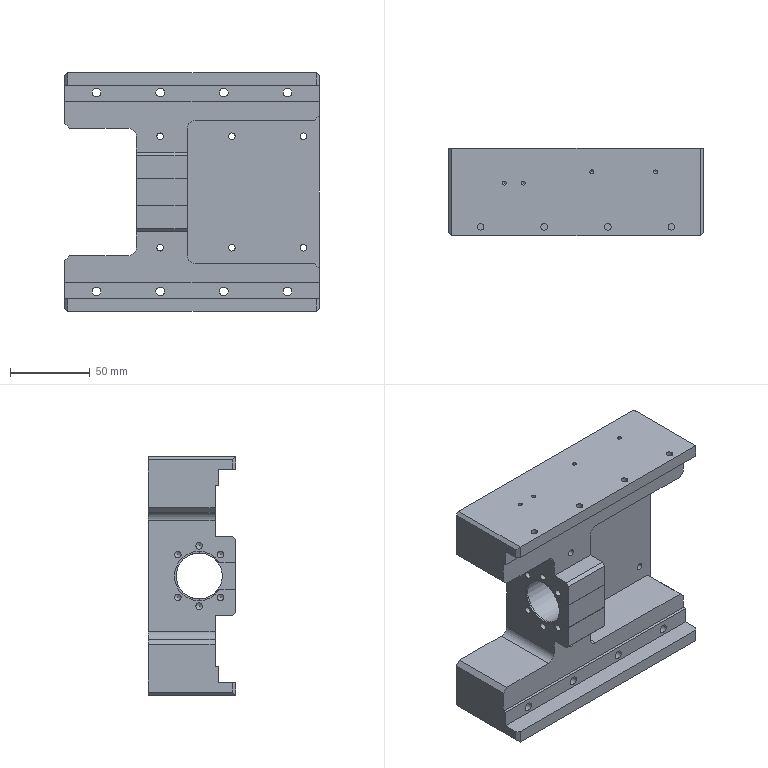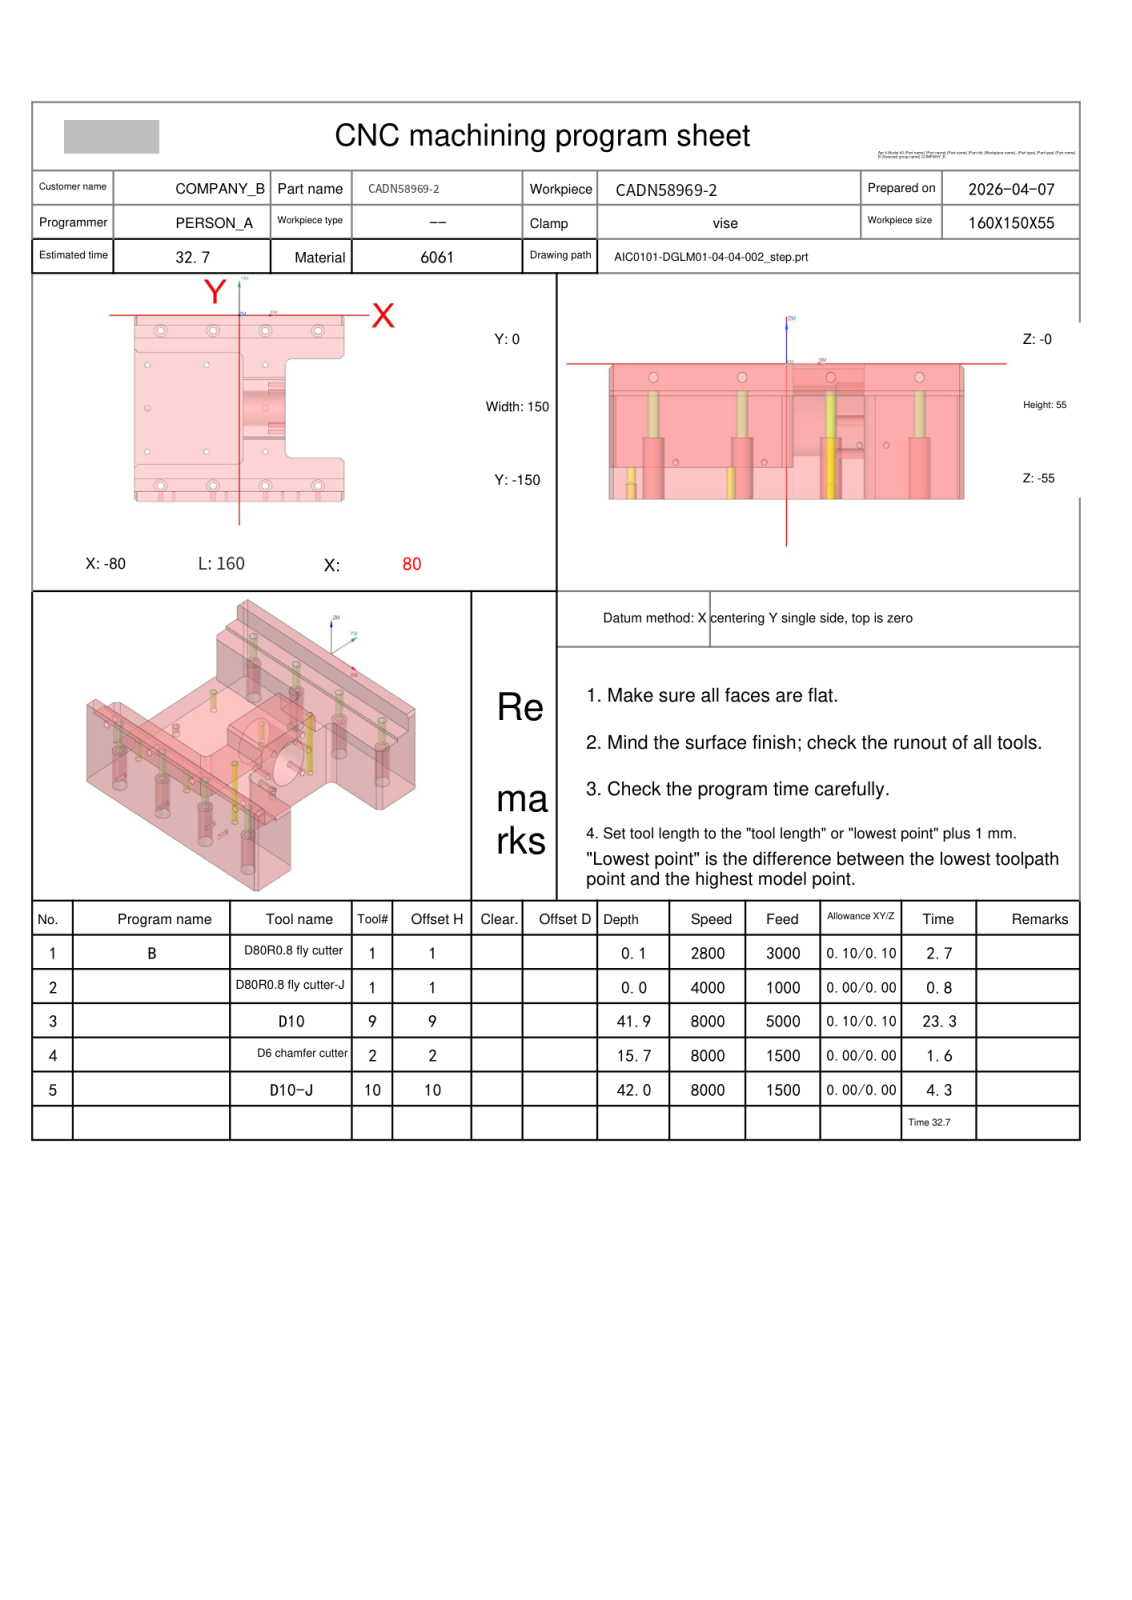NC program | NX | posted by the shop | part box 160 x 55 x 150 mm
Lines 13375 to 14160 of 14160:
N4 T02 M06
(D6 chamfer cutter D=6. R=0. H=02 ce=0.00 di=0.10)
G00 G90 G54 X20. Y-110. M03 S8000
G43 H02 Z20.
M08
G98 G81 X20. Y-110. Z-15.7 R-10. F1000.
Y-40.
G80
G00 Z20.
G00 G90 X78.792 Y-8.99 M03 S6500
Z20.
Z.13
G01 Z-1.2 F1500.
G03 X78.452 Y-8.915 I-.601 J-1.907
G01 X78.398 Y-8.905
X78.349 Y-8.928
X78.259 Y-8.966
X78. Y-9.
X-78.
X-78.259 Y-8.966
X-78.349 Y-8.929
X-78.398 Y-8.905
X-78.452 Y-8.915
G03 X-78.792 Y-8.991 I.261 J-1.983
G01 Z.13
G00 Z2.8
X-78.903 Y.41
G01 Z-1.2
X-78.866 Y.5
X-78.707 Y.707
X-78.5 Y.866
X-78.259 Y.966
X-78. Y1.
X0.0
X78.
X78.259 Y.966
X78.5 Y.866
X78.707 Y.707
X78.866 Y.5
X78.903 Y.41
Z2.8
G00 Z10.
X35.99 Y-51.208
Z.13
G01 Z-1.2
G03 X35.915 Y-51.548 I1.907 J-.601
G01 X35.905 Y-51.602
X35.928 Y-51.651
X35.966 Y-51.741
X36. Y-52.
Y-98.
X35.966 Y-98.259
X35.928 Y-98.349
X35.905 Y-98.398
X35.915 Y-98.452
G03 X35.99 Y-98.792 I1.983 J.261
G01 Z.13
G00 Z10.
X2.01
Z.13
G01 Z-1.2
G03 X2.085 Y-98.452 I-1.907 J.601
G01 X2.095 Y-98.398
X2.072 Y-98.349
X2.034 Y-98.259
X2. Y-98.
Y-75.
Y-52.
X2.034 Y-51.741
X2.072 Y-51.651
X2.095 Y-51.602
X2.085 Y-51.548
G03 X2.01 Y-51.208 I-1.983 J-.261
G01 Z.13
G00 Z10.
X78.903 Y-150.41
Z2.8
G01 Z-1.2
X78.866 Y-150.5
X78.707 Y-150.707
X78.5 Y-150.866
X78.259 Y-150.966
X78. Y-151.
X-78.
X-78.259 Y-150.966
X-78.5 Y-150.866
X-78.707 Y-150.707
X-78.866 Y-150.5
X-78.903 Y-150.41
Z2.8
G00 X-78.792 Y-141.01
Z.13
G01 Z-1.2
G03 X-78.452 Y-141.085 I.601 J1.907
G01 X-78.398 Y-141.095
X-78.349 Y-141.072
X-78.259 Y-141.034
X-78. Y-141.
X0.0
X78.
X78.259 Y-141.034
X78.349 Y-141.072
X78.398 Y-141.095
X78.452 Y-141.085
G03 X78.792 Y-141.01 I-.261 J1.983
G01 Z.13
G00 Z10.
X-81.068 Y-138.968
Z-2.305
G01 Z-12.2
X-81.008 Y-138.882
X-81. Y-138.852
Y-131.8
G02 X-80. Y-130.8 I1. J0.0
G01 X80.
G02 X81. Y-131.8 I0.0 J-1.
G01 Y-138.882
X81.005 Y-138.902
X81.045 Y-138.959
Z-2.292
G00 Z10.
X-59.172 Y-138.791
Z-1.81
G01 Z-12.2
G03 X-58.826 Y-138.749 I-.07 J1.999
G01 X-58.772 Y-138.74
X-58.733 Y-138.702
X-58.699 Y-138.671
G03 X-58.25 Y-137.5 I-1.301 J1.171
X-60. Y-135.75 I-1.75 J0.0
X-61.75 Y-137.5 I0.0 J-1.75
X-61.664 Y-138.041 I1.75 J0.0
G01 X-61.516 Y-138.375
X-61.301 Y-138.671
X-61.267 Y-138.702
X-61.232 Y-138.726
X-61.189 Y-138.76
X-61.135 Y-138.763
X-60.94 Y-138.772
X-60.786 Y-138.766
Z-1.835
G00 Z10.
X-19.172 Y-138.791
Z-1.81
G01 Z-12.2
G03 X-18.826 Y-138.749 I-.07 J1.999
G01 X-18.772 Y-138.74
X-18.733 Y-138.702
X-18.699 Y-138.671
G03 X-18.25 Y-137.5 I-1.301 J1.171
X-20. Y-135.75 I-1.75 J0.0
X-21.75 Y-137.5 I0.0 J-1.75
X-21.664 Y-138.041 I1.75 J0.0
G01 X-21.516 Y-138.375
X-21.301 Y-138.671
X-21.267 Y-138.702
X-21.232 Y-138.726
X-21.189 Y-138.76
X-21.135 Y-138.763
X-20.94 Y-138.772
X-20.786 Y-138.766
Z-1.835
G00 Z10.
X20.828 Y-138.791
Z-1.81
G01 Z-12.2
G03 X21.174 Y-138.749 I-.07 J1.999
G01 X21.228 Y-138.74
X21.267 Y-138.702
X21.301 Y-138.671
G03 X21.75 Y-137.5 I-1.301 J1.171
X20. Y-135.75 I-1.75 J0.0
X18.25 Y-137.5 I0.0 J-1.75
X18.336 Y-138.041 I1.75 J0.0
G01 X18.484 Y-138.375
X18.699 Y-138.671
X18.733 Y-138.702
X18.768 Y-138.726
X18.811 Y-138.76
X18.865 Y-138.763
X19.06 Y-138.772
X19.214 Y-138.766
Z-1.835
G00 Z10.
X60.828 Y-138.791
Z-1.81
G01 Z-12.2
G03 X61.174 Y-138.749 I-.07 J1.999
G01 X61.228 Y-138.74
X61.267 Y-138.702
X61.301 Y-138.671
G03 X61.75 Y-137.5 I-1.301 J1.171
X60. Y-135.75 I-1.75 J0.0
X58.25 Y-137.5 I0.0 J-1.75
X58.336 Y-138.041 I1.75 J0.0
G01 X58.484 Y-138.375
X58.699 Y-138.671
X58.733 Y-138.702
X58.768 Y-138.726
X58.811 Y-138.76
X58.865 Y-138.763
X59.06 Y-138.772
X59.214 Y-138.766
Z-1.835
G00 Z10.
X81.068 Y-11.032
Z-2.305
G01 Z-12.2
X81.008 Y-11.118
X81. Y-11.148
Y-18.2
G02 X80. Y-19.2 I-1. J0.0
G01 X-80.
G02 X-81. Y-18.2 I0.0 J1.
G01 Y-11.118
X-81.005 Y-11.098
X-81.045 Y-11.041
Z-2.292
G00 Z10.
X-60.828 Y-11.209
Z-1.81
G01 Z-12.2
G03 X-61.174 Y-11.251 I.07 J-1.999
G01 X-61.228 Y-11.26
X-61.267 Y-11.298
X-61.301 Y-11.329
G03 X-61.75 Y-12.5 I1.301 J-1.171
X-60. Y-14.25 I1.75 J0.0
X-58.25 Y-12.5 I0.0 J1.75
X-58.336 Y-11.959 I-1.75 J0.0
G01 X-58.484 Y-11.625
X-58.699 Y-11.329
X-58.733 Y-11.298
X-58.768 Y-11.274
X-58.811 Y-11.24
X-58.865 Y-11.237
X-59.06 Y-11.228
X-59.214 Y-11.234
Z-1.835
G00 Z10.
X-20.828 Y-11.209
Z-1.81
G01 Z-12.2
G03 X-21.174 Y-11.251 I.07 J-1.999
G01 X-21.228 Y-11.26
X-21.267 Y-11.298
X-21.301 Y-11.329
G03 X-21.75 Y-12.5 I1.301 J-1.171
X-20. Y-14.25 I1.75 J0.0
X-18.25 Y-12.5 I0.0 J1.75
X-18.336 Y-11.959 I-1.75 J0.0
G01 X-18.484 Y-11.625
X-18.699 Y-11.329
X-18.733 Y-11.298
X-18.768 Y-11.274
X-18.811 Y-11.24
X-18.865 Y-11.237
X-19.06 Y-11.228
X-19.214 Y-11.234
Z-1.835
G00 Z10.
X19.172 Y-11.209
Z-1.81
G01 Z-12.2
G03 X18.826 Y-11.251 I.07 J-1.999
G01 X18.772 Y-11.26
X18.733 Y-11.298
X18.699 Y-11.329
G03 X18.25 Y-12.5 I1.301 J-1.171
X20. Y-14.25 I1.75 J0.0
X21.75 Y-12.5 I0.0 J1.75
X21.664 Y-11.959 I-1.75 J0.0
G01 X21.516 Y-11.625
X21.301 Y-11.329
X21.267 Y-11.298
X21.232 Y-11.274
X21.189 Y-11.24
X21.135 Y-11.237
X20.94 Y-11.228
X20.786 Y-11.234
Z-1.835
G00 Z10.
X59.172 Y-11.209
Z-1.81
G01 Z-12.2
G03 X58.826 Y-11.251 I.07 J-1.999
G01 X58.772 Y-11.26
X58.733 Y-11.298
X58.699 Y-11.329
G03 X58.25 Y-12.5 I1.301 J-1.171
X59.636 Y-14.212 I1.75 J0.0
G01 X60. Y-14.25
G03 X61.75 Y-12.5 I0.0 J1.75
X61.516 Y-11.625 I-1.75 J0.0
G01 X61.301 Y-11.329
X61.267 Y-11.298
X61.232 Y-11.274
X61.189 Y-11.24
X61.135 Y-11.237
X60.94 Y-11.228
X60.786 Y-11.234
Z-1.835
G00 Z10.
X36.068 Y-103.009
Z-3.086
G01 Z-14.2
X36.008 Y-103.095
X36. Y-103.125
Y-110.
G03 X40. Y-114. I4. J0.0
G01 X77.
X77.259 Y-114.034
X77.5 Y-114.134
X77.707 Y-114.293
X80.707 Y-117.293
X80.866 Y-117.5
X80.966 Y-117.741
X81. Y-118.
Y-128.7
X81.008 Y-128.73
X81.068 Y-128.816
Z-12.669
G00 Z10.
X-81.068 Y-128.822
Z-12.669
G01 Z-14.2
X-81.008 Y-128.736
X-81. Y-128.706
Y-123.
X-80.966 Y-122.741
X-80.866 Y-122.5
X-80.707 Y-122.293
X-77.707 Y-119.293
X-77.5 Y-119.134
X-77.259 Y-119.034
X-77. Y-119.
X-2.
G03 X2. Y-115. I0.0 J4.
G01 Y-103.135
X1.992 Y-103.105
X1.932 Y-103.019
Z-3.096
G00 Z10.
X19.588 Y-110.926
Z-12.68
G01 Z-14.2
G03 X19.897 Y-111.086 I1.075 J1.687
G01 X19.946 Y-111.11
X20. Y-111.1
G03 X21.1 Y-110. I0.0 J1.1
X20. Y-108.9 I-1.1 J0.0
X18.9 Y-110. I0.0 J-1.1
X20. Y-111.1 I1.1 J0.0
G01 X20.054 Y-111.11
X20.103 Y-111.086
G03 X20.412 Y-110.926 I-.765 J1.848
G01 Z-12.68
G00 Z10.
X81.068 Y-21.184
Z-12.669
G01 Z-14.2
X81.008 Y-21.27
X81. Y-21.3
Y-32.
X80.966 Y-32.259
X80.866 Y-32.5
X80.707 Y-32.707
X77.707 Y-35.707
X77.5 Y-35.866
X77.259 Y-35.966
X77. Y-36.
X40.
G03 X36. Y-40. I0.0 J-4.
G01 Y-46.875
X36.008 Y-46.905
X36.068 Y-46.991
Z-3.086
G00 Z10.
X1.932 Y-46.981
Z-3.096
G01 Z-14.2
X1.992 Y-46.895
X2. Y-46.865
Y-35.
G03 X-2. Y-31. I-4. J0.0
G01 X-77.
X-77.259 Y-30.966
X-77.5 Y-30.866
X-77.707 Y-30.707
X-80.707 Y-27.707
X-80.866 Y-27.5
X-80.966 Y-27.259
X-81. Y-27.
Y-21.294
X-81.008 Y-21.264
X-81.068 Y-21.178
Z-12.669
G00 Z10.
X19.588 Y-40.926
Z-12.68
G01 Z-14.2
G03 X19.897 Y-41.086 I1.075 J1.687
G01 X19.946 Y-41.11
X20. Y-41.1
G03 X21.1 Y-40. I0.0 J1.1
X20. Y-38.9 I-1.1 J0.0
X18.9 Y-40. I0.0 J-1.1
X20. Y-41.1 I1.1 J0.0
G01 X20.054 Y-41.11
X20.103 Y-41.086
G03 X20.412 Y-40.926 I-.765 J1.848
G01 Z-12.68
G00 Z20.
G00 G90 X-81.9 Y-152.407 M03 S6500
Z20.
Z-1.2
G01 Z-2.7 F1500.
G03 X-80.7 Y-151.207 I0.0 J1.2
G01 Y-139.237
G03 X-81.516 Y-138.1 I-1.2 J0.0
G01 Z-1.2
G00 Z20.
Y-11.9
Z-1.2
G01 Z-2.7
G03 X-80.7 Y-10.763 I-.384 J1.137
G01 Y1.207
G03 X-81.9 Y2.407 I-1.2 J0.0
G01 Z-1.2
G00 Z20.
X81.9
Z-1.2
G01 Z-2.7
G03 X80.7 Y1.207 I0.0 J-1.2
G01 Y-10.763
G03 X81.516 Y-11.9 I1.2 J0.0
G01 Z-1.2
G00 Z20.
X-.9 Y-48.484
Z-1.2
G01 Z-2.7
G03 X.237 Y-49.3 I1.137 J.384
G01 X37.763
G03 X38.9 Y-48.484 I0.0 J1.2
G01 Z-1.2
G00 Z20.
Y-101.516
Z-1.2
G01 Z-2.7
G03 X37.763 Y-100.7 I-1.137 J-.384
G01 X.237
G03 X-.9 Y-101.516 I0.0 J-1.2
G01 Z-1.2
G00 Z20.
X81.516 Y-138.1
Z-1.2
G01 Z-2.7
G03 X80.7 Y-139.237 I.384 J-1.137
G01 Y-151.207
G03 X81.9 Y-152.407 I1.2 J0.0
G01 Z-1.2
G00 Z20.
G91 G28 Z0.0
M05
M09
G91 G28 Z0.0
M01
N5 T10 M06
(D10-J  D=10. R=0. H=10 ce=0.40 di=0.00)
G00 G90 G54 X-87. Y-128.801 M03 S7000
G43 H10 Z14.5
M08
Z-9.5
G01 Z-11. F1500.
G03 X-85. Y-130.8 I2. J.001
G01 X84.001
G02 X85. Y-131.799 I-.001 J-1.
G01 Y-132.701
G02 X84.001 Y-133.7 I-1. J.001
G01 X-84.1
G03 X-85. Y-134.6 I0.0 J-.9
G01 Y-135.6
G03 X-84. Y-136.6 I1. J0.0
G01 X85.
G03 X87. Y-134.6 I0.0 J2.
G01 Z-9.5
G00 Z14.5
X-4. Y-107.401
Z-11.5
G01 Z-13.
X0.0
G03 X-2. Y-105.401 I-2. J0.0
G01 X39.1
G02 X40. Y-106.301 I0.0 J-.9
G01 Y-108.601
G02 X39. Y-109.601 I-1. J0.0
G01 X-1.1
G03 X-2. Y-110.501 I0.0 J-.9
G01 Y-112.801
G03 X-1. Y-113.801 I1. J0.0
G01 X82.458
G02 X83.164 Y-114.093 I-.001 J-1.
G01 X84.707 Y-115.636
G02 X85. Y-116.343 I-.707 J-.707
G01 Y-117.001
G02 X84.001 Y-118. I-1. J.001
G01 X-81.658
G03 X-82.364 Y-118.293 I.001 J-1.
G01 X-84.707 Y-120.636
G03 X-85. Y-121.343 I.707 J-.707
G01 Y-121.401
G03 X-84.201 Y-122.2 I.8 J.001
G01 X84.1
G02 X85. Y-123.1 I0.0 J-.9
G01 Y-125.4
G02 X84. Y-126.4 I-1. J0.0
G01 X-85.
G02 X-87. Y-124.4 I0.0 J2.
G01 Z-11.5
G00 Z14.5
Y-25.601
Z-11.5
G01 Z-13.
X-83.
G03 X-85. Y-23.601 I-2. J0.0
G01 X84.1
G02 X85. Y-24.501 I0.0 J-.9
G01 Y-26.801
G02 X84. Y-27.801 I-1. J0.0
G01 X-84.201
G03 X-85. Y-28.6 I.001 J-.8
G01 Y-28.657
G03 X-84.707 Y-29.364 I1. J0.0
G01 X-82.363 Y-31.708
G03 X-81.657 Y-32.001 I.706 J.708
G01 X84.001
G02 X85. Y-33. I-.001 J-1.
G01 Y-33.657
G02 X84.707 Y-34.364 I-1. J0.0
G01 X83.163 Y-35.908
G02 X82.457 Y-36.2 I-.707 J.708
G01 X-1.1
G03 X-2. Y-37.1 I0.0 J-.9
G01 Y-39.4
G03 X-1. Y-40.4 I1. J0.0
G01 X39.1
G02 X40. Y-41.3 I0.0 J-.9
G01 Y-43.6
G02 X39. Y-44.6 I-1. J0.0
G01 X-2.
G02 X-4. Y-42.6 I0.0 J2.
G01 Z-11.5
G00 Z14.5
X87. Y-21.2
Z-9.5
G01 Z-11.
G03 X85. Y-19.2 I-2. J0.0
G01 X-84.
G02 X-85. Y-18.2 I0.0 J1.
G01 Y-17.2
G02 X-84.1 Y-16.3 I.9 J0.0
G01 X84.1
G03 X85. Y-15.4 I0.0 J.9
G01 Y-14.4
G03 X84. Y-13.4 I-1. J0.0
G01 X-85.
G03 X-87. Y-15.4 I0.0 J-2.
G01 Z-9.5
G00 Z14.5
G00 G90 X-87. Y-72.252 M03 S7000
Z14.5
Z-40.5
G01 Z-42. F1500.
X-83.098
G02 X-81.101 Y-70.353 I1.997 J-.101
G01 X-81. Y-70.356
G03 X-79.237 Y-70.4 I1.763 J34.956
G01 X-38.395
G02 X-37.4 Y-71.395 I-.005 J-1.
G01 Y-78.605
G02 X-38.395 Y-79.6 I-1. J.005
G01 X-79.24
G03 X-80.023 Y-79.609 I.004 J-35.
X-81. Y-80.608 I.023 J-1.
G01 Y-83.713
G03 X-80.1 Y-84.612 I.9 J0.0
G01 X-80.075
G02 X-79.24 Y-84.6 I.839 J-29.988
G01 X-33.395
G03 X-32.4 Y-83.605 I-.005 J1.
G01 Y-66.395
G03 X-33.395 Y-65.4 I-1. J-.005
G01 X-79.237
G02 X-80.027 Y-65.39 I0.0 J30.
X-81. Y-64.39 I.027 J1.
G01 Y-61.285
G02 X-80.1 Y-60.386 I.9 J-.001
G01 X-80.07
G03 X-79.237 Y-60.4 I.834 J24.986
G01 X-28.396
G02 X-27.4 Y-61.396 I-.004 J-1.
G01 Y-88.604
G02 X-28.396 Y-89.6 I-1. J.004
G01 X-79.239
G03 X-80.032 Y-89.613 I.003 J-25.
X-81. Y-90.612 I.032 J-.999
G01 Y-93.718
G03 X-80.1 Y-94.618 I.9 J.001
G01 X-80.063 Y-94.617
G02 X-79.239 Y-94.6 I.827 J-19.983
G01 X-23.396
G03 X-22.4 Y-93.604 I-.004 J1.
G01 Y-56.396
G03 X-23.396 Y-55.4 I-1. J-.004
G01 X-79.237
G02 X-80.041 Y-55.384 I0.0 J20.
X-81. Y-54.385 I.041 J.999
G01 Y-51.276
G02 X-80.1 Y-50.377 I.9 J-.001
G01 X-80.052 Y-50.378
G03 X-79.237 Y-50.4 I.815 J14.978
G01 X-18.396
G02 X-17.4 Y-51.396 I-.004 J-1.
G01 Y-98.604
G02 X-18.396 Y-99.6 I-1. J.004
G01 X-79.238
G03 X-80.055 Y-99.622 I.002 J-15.
X-81. Y-100.62 I.055 J-.998
G01 Y-103.844
G03 X-80.2 Y-104.643 I.8 J.001
G01 X-80.129 Y-104.64
G02 X-79.238 Y-104.6 I.892 J-9.96
G01 X-13.397
G03 X-12.4 Y-103.603 I-.003 J1.
G01 Y-46.397
G03 X-13.397 Y-45.4 I-1. J-.003
G01 X-79.237
G02 X-80.085 Y-45.364 I0.0 J10.
X-81. Y-44.368 I.085 J.996
G01 Y-40.999
G02 X-80.3 Y-40.3 I.7 J-.001
G01 X-80.17 Y-40.312
G03 X-79.237 Y-40.4 I.933 J4.912
G01 X-8.397
G02 X-7.4 Y-41.397 I-.003 J-1.
G01 Y-108.603
G02 X-8.397 Y-109.6 I-1. J.003
G01 X-79.237
G03 X-80.438 Y-109.747 I0.0 J-5.
X-81.154 Y-110.424 I.241 J-.971
G01 X-82.663 Y-115.364
G03 X-82.707 Y-115.656 I.956 J-.292
X-81.707 Y-116.656 I1. J0.0
X-81. Y-116.363 I0.0 J1.
G01 X-79.237 Y-114.6
X-3.397
G03 X-2.4 Y-113.603 I-.003 J1.
G01 Y-36.397
G03 X-3.397 Y-35.4 I-1. J-.003
G01 X-79.237
X-81. Y-33.637
G03 X-82.414 Y-33.051 I-1.414 J-1.414
X-83.828 Y-33.637 I0.0 J-2.
G01 X-87. Y-36.808
Z-40.5
G00 Z14.5
G00 G90 X87. Y-15.199 M03 S8000
Z14.5
Z-10.
G01 Z-11. F1000.
G41 D10
Y-14.999
G03 X85. Y-13. I-2. J-.001
G01 X-85.
G03 X-87. Y-14.999 I0.0 J-2.
G01 G40 Y-15.199
Z-10.
G00 Z3.
Y-134.801
Z-10.
G01 Z-11.
G41 D10
Y-135.001
G03 X-85. Y-137. I2. J.001
G01 X85.
G03 X87. Y-135.001 I0.0 J2.
G01 G40 Y-134.801
Z-10.
G00 Z14.5
G00 G90 X-4. Y-42.801 M03 S8000
Z14.5
Z-12.
G01 Z-13. F1000.
G41 D10
Y-43.001
G03 X-2. Y-45. I2. J.001
G01 X40.
G03 X42. Y-43.001 I0.0 J2.
G01 G40 Y-42.801
Z-12.
G00 X87. Y-25.399
G01 Z-13.
G41 D10
Y-25.199
G03 X85. Y-23.2 I-2. J-.001
G01 X-85.
G03 X-87. Y-25.199 I0.0 J-2.
G01 G40 Y-25.399
Z-12.
G00 Z3.
Y-124.601
Z-12.
G01 Z-13.
G41 D10
Y-124.801
G03 X-85. Y-126.8 I2. J.001
G01 X85.
G03 X87. Y-124.801 I0.0 J2.
G01 G40 Y-124.601
Z-12.
G00 X42. Y-107.199
G01 Z-13.
G41 D10
Y-106.999
G03 X40. Y-105. I-2. J-.001
G01 X-2.
G03 X-4. Y-106.999 I0.0 J-2.
G01 G40 Y-107.199
Z-12.
G00 Z14.5
G00 G90 X-87.191 Y-121.368 M03 S8000
Z14.5
Z-13.
G01 Z-14. F1000.
G41 D10
X-87. Y-121.427
G03 X-86.414 Y-121.515 I.586 J1.912
X-85. Y-120.929 I0.0 J2.
G01 X-79.071 Y-115.
X-2.
Y-35.
X-79.071
X-85. Y-29.071
G03 X-86.414 Y-28.485 I-1.414 J-1.414
X-87. Y-28.573 I0.0 J-2.
G01 G40 X-87.191 Y-28.632
Z-13.
G00 Y-121.368
Z-27.
G01 Z-28.
G41 D10
X-87. Y-121.427
G03 X-86.414 Y-121.515 I.586 J1.912
X-85. Y-120.929 I0.0 J2.
G01 X-79.071 Y-115.
X-2.
Y-35.
X-79.071
X-85. Y-29.071
G03 X-86.414 Y-28.485 I-1.414 J-1.414
X-87. Y-28.573 I0.0 J-2.
G01 G40 X-87.191 Y-28.632
Z-27.
G00 Y-121.368
Z-41.
G01 Z-42.
G41 D10
X-87. Y-121.427
G03 X-86.414 Y-121.515 I.586 J1.912
X-85. Y-120.929 I0.0 J2.
G01 X-79.071 Y-115.
X-2.
Y-35.
X-79.071
X-85. Y-29.071
G03 X-86.414 Y-28.485 I-1.414 J-1.414
X-87. Y-28.573 I0.0 J-2.
G01 G40 X-87.191 Y-28.632
Z-41.
G00 Z14.5
M05
M09
G91 G28 Z0.0
G91 G28 Y0.0
M30
%